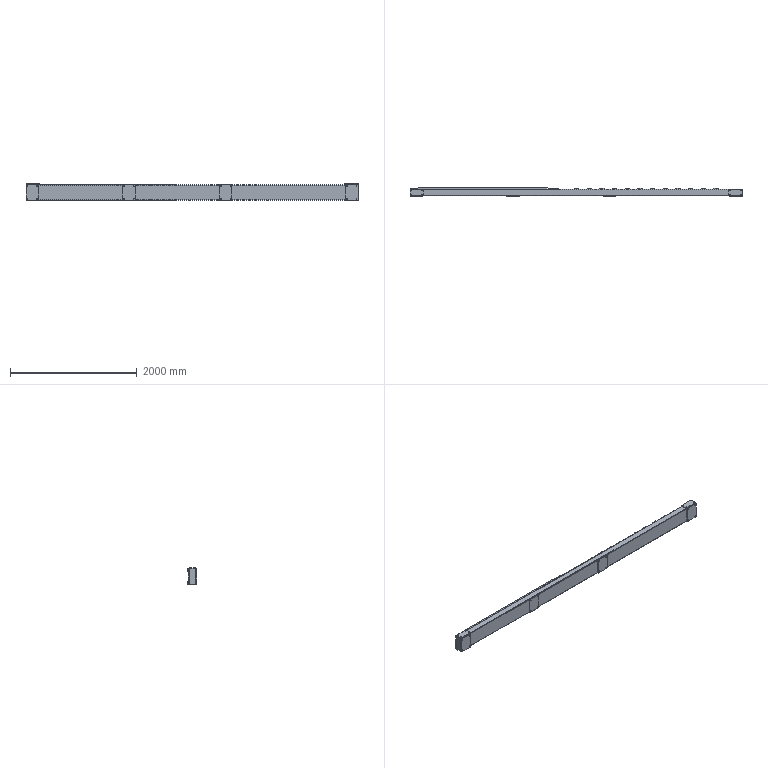Part | SolidWorks | features ICE 9, HoleWzd 7, DeleteBody 1, MirrorSolid 1, WeldCornerFeat 1, WeldMemberFeat 1, WeldmentFeature 1 | 25 solids | 732 faces | box 5240 x 145 x 265 mm | volume 27147429 mm3 | cylinder 328 | plane 236 | cone 168 | commonest cylinder face diameters 6.8 x104 10.2 x96 5 x68 8.5 x32 8 x12 4.2 x8